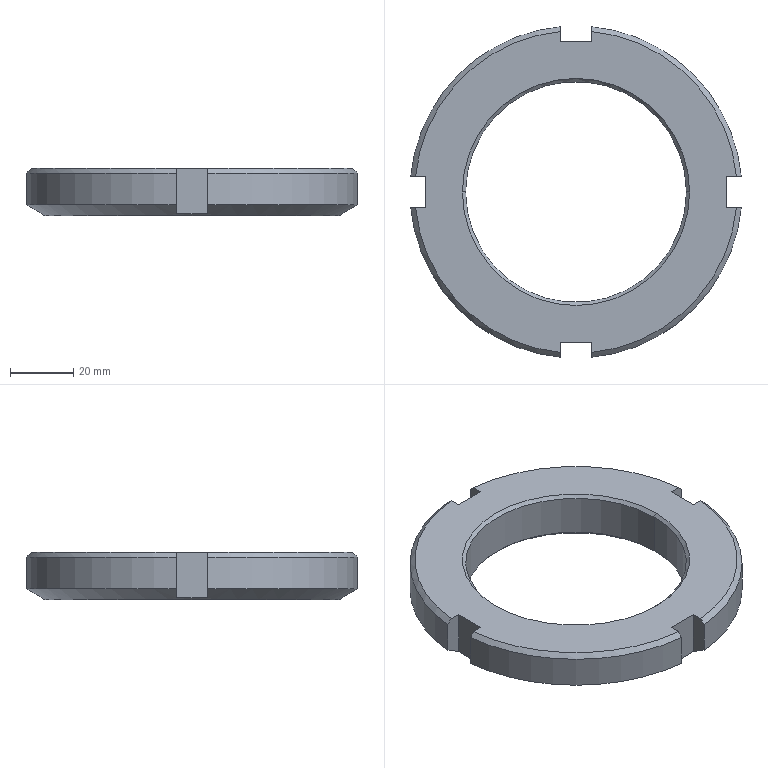Part | SolidWorks | features Chamfer 3, CirPattern 1, Cut 1, Extrusion 1 | 1 solid | 30 faces | box 104.523 x 104.523 x 15 mm | volume 66046 mm3 | plane 14 | cone 10 | cylinder 6 | commonest cylinder face diameters 105 x4 69.835 x2
STEP:
#1=CARTESIAN_POINT('',(-34.917,0.,14.));
#2=VERTEX_POINT('',#1);
#3=CARTESIAN_POINT('',(34.917,0.,14.));
#4=VERTEX_POINT('',#3);
#5=CARTESIAN_POINT('',(0.,0.,14.));
#6=DIRECTION('',(0.,0.,1.));
#7=DIRECTION('',(1.,0.,0.));
#8=AXIS2_PLACEMENT_3D('',#5,#6,#7);
#9=CIRCLE('',#8,34.917);
#10=EDGE_CURVE('',#2,#4,#9,.T.);
#11=ORIENTED_EDGE('',*,*,#10,.F.);
#12=CARTESIAN_POINT('',(-35.918,0.,15.));
#13=VERTEX_POINT('',#12);
#14=CARTESIAN_POINT('',(-34.917,0.,14.));
#15=DIRECTION('',(-0.7071,0.,0.7071));
#16=VECTOR('',#15,1000.);
#17=LINE('',#14,#16);
#18=EDGE_CURVE('',#2,#13,#17,.T.);
#19=ORIENTED_EDGE('',*,*,#18,.T.);
#20=CARTESIAN_POINT('',(35.918,0.,15.));
#21=VERTEX_POINT('',#20);
#22=CARTESIAN_POINT('',(0.,0.,15.));
#23=DIRECTION('',(0.,0.,-1.));
#24=DIRECTION('',(1.,0.,0.));
#25=AXIS2_PLACEMENT_3D('',#22,#23,#24);
#26=CIRCLE('',#25,35.918);
#27=EDGE_CURVE('',#21,#13,#26,.T.);
#28=ORIENTED_EDGE('',*,*,#27,.F.);
#29=CARTESIAN_POINT('',(34.917,0.,14.));
#30=DIRECTION('',(0.7071,0.,0.7071));
#31=VECTOR('',#30,1000.);
#32=LINE('',#29,#31);
#33=EDGE_CURVE('',#4,#21,#32,.T.);
#34=ORIENTED_EDGE('',*,*,#33,.F.);
#35=EDGE_LOOP('',(#11,#19,#28,#34));
#36=FACE_OUTER_BOUND('',#35,.T.);
#37=CARTESIAN_POINT('',(0.,0.,14.));
#38=DIRECTION('',(0.,0.,1.));
#39=DIRECTION('',(1.,0.,0.));
#40=AXIS2_PLACEMENT_3D('',#37,#38,#39);
#41=CONICAL_SURFACE('',#40,34.917,0.7854);
#42=ADVANCED_FACE('',(#36),#41,.F.);
#43=CARTESIAN_POINT('',(34.917,0.,1.));
#44=VERTEX_POINT('',#43);
#45=CARTESIAN_POINT('',(-34.917,0.,1.));
#46=VERTEX_POINT('',#45);
#47=CARTESIAN_POINT('',(0.,0.,1.));
#48=DIRECTION('',(0.,0.,-1.));
#49=DIRECTION('',(1.,0.,0.));
#50=AXIS2_PLACEMENT_3D('',#47,#48,#49);
#51=CIRCLE('',#50,34.917);
#52=EDGE_CURVE('',#44,#46,#51,.T.);
#53=ORIENTED_EDGE('',*,*,#52,.F.);
#54=CARTESIAN_POINT('',(35.918,0.,0.));
#55=VERTEX_POINT('',#54);
#56=CARTESIAN_POINT('',(35.918,0.,0.));
#57=DIRECTION('',(0.7071,0.,-0.7071));
#58=VECTOR('',#57,1000.);
#59=LINE('',#56,#58);
#60=EDGE_CURVE('',#44,#55,#59,.T.);
#61=ORIENTED_EDGE('',*,*,#60,.T.);
#62=CARTESIAN_POINT('',(-35.918,0.,0.));
#63=VERTEX_POINT('',#62);
#64=CARTESIAN_POINT('',(0.,0.,0.));
#65=DIRECTION('',(0.,0.,1.));
#66=DIRECTION('',(1.,0.,0.));
#67=AXIS2_PLACEMENT_3D('',#64,#65,#66);
#68=CIRCLE('',#67,35.918);
#69=EDGE_CURVE('',#63,#55,#68,.T.);
#70=ORIENTED_EDGE('',*,*,#69,.F.);
#71=CARTESIAN_POINT('',(-35.918,0.,0.));
#72=DIRECTION('',(-0.7071,0.,-0.7071));
#73=VECTOR('',#72,1000.);
#74=LINE('',#71,#73);
#75=EDGE_CURVE('',#46,#63,#74,.T.);
#76=ORIENTED_EDGE('',*,*,#75,.F.);
#77=EDGE_LOOP('',(#53,#61,#70,#76));
#78=FACE_OUTER_BOUND('',#77,.T.);
#79=CARTESIAN_POINT('',(0.,0.,0.));
#80=DIRECTION('',(0.,0.,-1.));
#81=DIRECTION('',(-1.,0.,0.));
#82=AXIS2_PLACEMENT_3D('',#79,#80,#81);
#83=CONICAL_SURFACE('',#82,35.918,0.7854);
#84=ADVANCED_FACE('',(#78),#83,.F.);
#85=CARTESIAN_POINT('',(-46.5,0.,0.));
#86=VERTEX_POINT('',#85);
#87=CARTESIAN_POINT('',(46.5,0.,0.));
#88=VERTEX_POINT('',#87);
#89=CARTESIAN_POINT('',(0.,0.,0.));
#90=DIRECTION('',(0.,0.,-1.));
#91=DIRECTION('',(1.,0.,0.));
#92=AXIS2_PLACEMENT_3D('',#89,#90,#91);
#93=CIRCLE('',#92,46.5);
#94=EDGE_CURVE('',#86,#88,#93,.T.);
#95=ORIENTED_EDGE('',*,*,#94,.F.);
#96=CARTESIAN_POINT('',(-47.511,0.,0.5839));
#97=VERTEX_POINT('',#96);
#98=CARTESIAN_POINT('',(-52.5,0.,3.464));
#99=DIRECTION('',(-0.866,0.,0.5));
#100=VECTOR('',#99,1000.);
#101=LINE('',#98,#100);
#102=EDGE_CURVE('',#86,#97,#101,.T.);
#103=ORIENTED_EDGE('',*,*,#102,.T.);
#104=CARTESIAN_POINT('',(-47.511,5.,0.7354));
#105=VERTEX_POINT('',#104);
#106=CARTESIAN_POINT('',(-47.511,5.,0.7354));
#107=CARTESIAN_POINT('',(-47.511,3.337,0.6349));
#108=CARTESIAN_POINT('',(-47.511,1.671,0.5839));
#109=CARTESIAN_POINT('',(-47.511,0.,0.5839));
#110=B_SPLINE_CURVE_WITH_KNOTS('',3,(#106,#107,#108,#109),.UNSPECIFIED.,.F.,.F.,(4,4),(0.01217,0.01717),.UNSPECIFIED.);
#111=EDGE_CURVE('',#105,#97,#110,.T.);
#112=ORIENTED_EDGE('',*,*,#111,.F.);
#113=CARTESIAN_POINT('',(-52.261,5.,3.464));
#114=VERTEX_POINT('',#113);
#115=CARTESIAN_POINT('',(-52.261,5.,3.464));
#116=CARTESIAN_POINT('',(-51.988,5.,3.307));
#117=CARTESIAN_POINT('',(-51.714,5.,3.15));
#118=CARTESIAN_POINT('',(-51.441,5.,2.993));
#119=CARTESIAN_POINT('',(-50.131,5.,2.24));
#120=CARTESIAN_POINT('',(-48.821,5.,1.488));
#121=CARTESIAN_POINT('',(-47.511,5.,0.7354));
#122=B_SPLINE_CURVE_WITH_KNOTS('',3,(#115,#116,#117,#118,#119,#120,#121),.UNSPECIFIED.,.F.,.F.,(4,3,4),(0.01027,0.01122,0.01575),.UNSPECIFIED.);
#123=EDGE_CURVE('',#114,#105,#122,.T.);
#124=ORIENTED_EDGE('',*,*,#123,.F.);
#125=CARTESIAN_POINT('',(-5.,52.261,3.464));
#126=VERTEX_POINT('',#125);
#127=CARTESIAN_POINT('',(0.,0.,3.464));
#128=DIRECTION('',(0.,0.,1.));
#129=DIRECTION('',(1.,0.,0.));
#130=AXIS2_PLACEMENT_3D('',#127,#128,#129);
#131=CIRCLE('',#130,52.5);
#132=EDGE_CURVE('',#126,#114,#131,.T.);
#133=ORIENTED_EDGE('',*,*,#132,.F.);
#134=CARTESIAN_POINT('',(-5.,47.511,0.7354));
#135=VERTEX_POINT('',#134);
#136=CARTESIAN_POINT('',(-5.,47.511,0.7354));
#137=CARTESIAN_POINT('',(-5.,47.679,0.8316));
#138=CARTESIAN_POINT('',(-5.,47.847,0.9279));
#139=CARTESIAN_POINT('',(-5.,48.014,1.024));
#140=CARTESIAN_POINT('',(-5.,49.43,1.837));
#141=CARTESIAN_POINT('',(-5.,50.846,2.651));
#142=CARTESIAN_POINT('',(-5.,52.261,3.464));
#143=B_SPLINE_CURVE_WITH_KNOTS('',3,(#136,#137,#138,#139,#140,#141,#142),.UNSPECIFIED.,.F.,.F.,(4,3,4),(0.01064,0.01122,0.01612),.UNSPECIFIED.);
#144=EDGE_CURVE('',#135,#126,#143,.T.);
#145=ORIENTED_EDGE('',*,*,#144,.F.);
#146=CARTESIAN_POINT('',(5.,47.511,0.7354));
#147=VERTEX_POINT('',#146);
#148=CARTESIAN_POINT('',(5.,47.511,0.7354));
#149=CARTESIAN_POINT('',(3.341,47.511,0.6351));
#150=CARTESIAN_POINT('',(1.678,47.511,0.5841));
#151=CARTESIAN_POINT('',(-0.8227,47.511,0.5838));
#152=CARTESIAN_POINT('',(-1.657,47.511,0.5964));
#153=CARTESIAN_POINT('',(-3.328,47.511,0.6469));
#154=CARTESIAN_POINT('',(-4.165,47.511,0.685));
#155=CARTESIAN_POINT('',(-5.,47.511,0.7354));
#156=B_SPLINE_CURVE_WITH_KNOTS('',3,(#148,#149,#150,#151,#152,#153,#154,#155),.UNSPECIFIED.,.F.,.F.,(4,2,2,4),(0.01217,0.01715,0.01965,0.02214),.UNSPECIFIED.);
#157=EDGE_CURVE('',#147,#135,#156,.T.);
#158=ORIENTED_EDGE('',*,*,#157,.F.);
#159=CARTESIAN_POINT('',(5.,52.261,3.464));
#160=VERTEX_POINT('',#159);
#161=CARTESIAN_POINT('',(5.,52.261,3.464));
#162=CARTESIAN_POINT('',(5.,50.846,2.651));
#163=CARTESIAN_POINT('',(5.,49.43,1.837));
#164=CARTESIAN_POINT('',(5.,48.014,1.024));
#165=CARTESIAN_POINT('',(5.,47.847,0.9279));
#166=CARTESIAN_POINT('',(5.,47.679,0.8316));
#167=CARTESIAN_POINT('',(5.,47.511,0.7354));
#168=B_SPLINE_CURVE_WITH_KNOTS('',3,(#161,#162,#163,#164,#165,#166,#167),.UNSPECIFIED.,.F.,.F.,(4,3,4),(0.006321,0.01122,0.0118),.UNSPECIFIED.);
#169=EDGE_CURVE('',#160,#147,#168,.T.);
#170=ORIENTED_EDGE('',*,*,#169,.F.);
#171=CARTESIAN_POINT('',(52.261,5.,3.464));
#172=VERTEX_POINT('',#171);
#173=CARTESIAN_POINT('',(0.,0.,3.464));
#174=DIRECTION('',(0.,0.,1.));
#175=DIRECTION('',(1.,0.,0.));
#176=AXIS2_PLACEMENT_3D('',#173,#174,#175);
#177=CIRCLE('',#176,52.5);
#178=EDGE_CURVE('',#172,#160,#177,.T.);
#179=ORIENTED_EDGE('',*,*,#178,.F.);
#180=CARTESIAN_POINT('',(47.511,5.,0.7354));
#181=VERTEX_POINT('',#180);
#182=CARTESIAN_POINT('',(47.511,5.,0.7354));
#183=CARTESIAN_POINT('',(47.679,5.,0.8316));
#184=CARTESIAN_POINT('',(47.847,5.,0.9279));
#185=CARTESIAN_POINT('',(48.014,5.,1.024));
#186=CARTESIAN_POINT('',(49.43,5.,1.837));
#187=CARTESIAN_POINT('',(50.846,5.,2.651));
#188=CARTESIAN_POINT('',(52.261,5.,3.464));
#189=B_SPLINE_CURVE_WITH_KNOTS('',3,(#182,#183,#184,#185,#186,#187,#188),.UNSPECIFIED.,.F.,.F.,(4,3,4),(0.01064,0.01122,0.01612),.UNSPECIFIED.);
#190=EDGE_CURVE('',#181,#172,#189,.T.);
#191=ORIENTED_EDGE('',*,*,#190,.F.);
#192=CARTESIAN_POINT('',(47.511,0.,0.5839));
#193=VERTEX_POINT('',#192);
#194=CARTESIAN_POINT('',(47.511,0.,0.5839));
#195=CARTESIAN_POINT('',(47.511,1.671,0.5839));
#196=CARTESIAN_POINT('',(47.511,3.337,0.6349));
#197=CARTESIAN_POINT('',(47.511,5.,0.7354));
#198=B_SPLINE_CURVE_WITH_KNOTS('',3,(#194,#195,#196,#197),.UNSPECIFIED.,.F.,.F.,(4,4),(0.0247,0.02971),.UNSPECIFIED.);
#199=EDGE_CURVE('',#193,#181,#198,.T.);
#200=ORIENTED_EDGE('',*,*,#199,.F.);
#201=CARTESIAN_POINT('',(52.5,0.,3.464));
#202=DIRECTION('',(0.866,0.,0.5));
#203=VECTOR('',#202,1000.);
#204=LINE('',#201,#203);
#205=EDGE_CURVE('',#88,#193,#204,.T.);
#206=ORIENTED_EDGE('',*,*,#205,.F.);
#207=EDGE_LOOP('',(#95,#103,#112,#124,#133,#145,#158,#170,#179,#191,#200,#206));
#208=FACE_OUTER_BOUND('',#207,.T.);
#209=CARTESIAN_POINT('',(0.,0.,3.464));
#210=DIRECTION('',(0.,0.,1.));
#211=DIRECTION('',(1.,0.,0.));
#212=AXIS2_PLACEMENT_3D('',#209,#210,#211);
#213=CONICAL_SURFACE('',#212,52.5,1.047);
#214=ADVANCED_FACE('',(#208),#213,.T.);
#215=ORIENTED_EDGE('',*,*,#10,.T.);
#216=CARTESIAN_POINT('',(34.917,0.,15.));
#217=DIRECTION('',(0.,0.,-1.));
#218=VECTOR('',#217,1000.);
#219=LINE('',#216,#218);
#220=EDGE_CURVE('',#4,#44,#219,.T.);
#221=ORIENTED_EDGE('',*,*,#220,.T.);
#222=ORIENTED_EDGE('',*,*,#52,.T.);
#223=CARTESIAN_POINT('',(-34.917,0.,15.));
#224=DIRECTION('',(0.,0.,-1.));
#225=VECTOR('',#224,1000.);
#226=LINE('',#223,#225);
#227=EDGE_CURVE('',#2,#46,#226,.T.);
#228=ORIENTED_EDGE('',*,*,#227,.F.);
#229=EDGE_LOOP('',(#215,#221,#222,#228));
#230=FACE_OUTER_BOUND('',#229,.T.);
#231=CARTESIAN_POINT('',(0.,0.,15.));
#232=DIRECTION('',(0.,0.,-1.));
#233=DIRECTION('',(-1.,0.,0.));
#234=AXIS2_PLACEMENT_3D('',#231,#232,#233);
#235=CYLINDRICAL_SURFACE('',#234,34.917);
#236=ADVANCED_FACE('',(#230),#235,.F.);
#237=CARTESIAN_POINT('',(5.,52.261,13.5));
#238=VERTEX_POINT('',#237);
#239=CARTESIAN_POINT('',(52.261,5.,13.5));
#240=VERTEX_POINT('',#239);
#241=CARTESIAN_POINT('',(0.,0.,13.5));
#242=DIRECTION('',(0.,0.,-1.));
#243=DIRECTION('',(1.,0.,0.));
#244=AXIS2_PLACEMENT_3D('',#241,#242,#243);
#245=CIRCLE('',#244,52.5);
#246=EDGE_CURVE('',#238,#240,#245,.T.);
#247=ORIENTED_EDGE('',*,*,#246,.T.);
#248=CARTESIAN_POINT('',(52.261,5.,0.));
#249=DIRECTION('',(0.,0.,1.));
#250=VECTOR('',#249,1000.);
#251=LINE('',#248,#250);
#252=EDGE_CURVE('',#172,#240,#251,.T.);
#253=ORIENTED_EDGE('',*,*,#252,.F.);
#254=ORIENTED_EDGE('',*,*,#178,.T.);
#255=CARTESIAN_POINT('',(5.,52.261,0.));
#256=DIRECTION('',(0.,0.,1.));
#257=VECTOR('',#256,1000.);
#258=LINE('',#255,#257);
#259=EDGE_CURVE('',#160,#238,#258,.T.);
#260=ORIENTED_EDGE('',*,*,#259,.T.);
#261=EDGE_LOOP('',(#247,#253,#254,#260));
#262=FACE_OUTER_BOUND('',#261,.T.);
#263=CARTESIAN_POINT('',(0.,0.,15.));
#264=DIRECTION('',(0.,0.,-1.));
#265=DIRECTION('',(-1.,0.,0.));
#266=AXIS2_PLACEMENT_3D('',#263,#264,#265);
#267=CYLINDRICAL_SURFACE('',#266,52.5);
#268=ADVANCED_FACE('',(#262),#267,.T.);
#269=CARTESIAN_POINT('',(50.754,5.,15.));
#270=VERTEX_POINT('',#269);
#271=CARTESIAN_POINT('',(52.261,5.,13.5));
#272=CARTESIAN_POINT('',(51.838,5.,13.921));
#273=CARTESIAN_POINT('',(51.415,5.,14.343));
#274=CARTESIAN_POINT('',(50.992,5.,14.764));
#275=CARTESIAN_POINT('',(50.912,5.,14.843));
#276=CARTESIAN_POINT('',(50.833,5.,14.921));
#277=CARTESIAN_POINT('',(50.754,5.,15.));
#278=B_SPLINE_CURVE_WITH_KNOTS('',3,(#271,#272,#273,#274,#275,#276,#277),.UNSPECIFIED.,.F.,.F.,(4,3,4),(0.00787,0.009662,0.009997),.UNSPECIFIED.);
#279=EDGE_CURVE('',#240,#270,#278,.T.);
#280=ORIENTED_EDGE('',*,*,#279,.F.);
#281=ORIENTED_EDGE('',*,*,#246,.F.);
#282=CARTESIAN_POINT('',(5.,50.754,15.));
#283=VERTEX_POINT('',#282);
#284=CARTESIAN_POINT('',(5.,50.754,15.));
#285=CARTESIAN_POINT('',(5.,50.833,14.921));
#286=CARTESIAN_POINT('',(5.,50.912,14.843));
#287=CARTESIAN_POINT('',(5.,50.992,14.764));
#288=CARTESIAN_POINT('',(5.,51.415,14.343));
#289=CARTESIAN_POINT('',(5.,51.838,13.921));
#290=CARTESIAN_POINT('',(5.,52.261,13.5));
#291=B_SPLINE_CURVE_WITH_KNOTS('',3,(#284,#285,#286,#287,#288,#289,#290),.UNSPECIFIED.,.F.,.F.,(4,3,4),(0.009327,0.009662,0.01145),.UNSPECIFIED.);
#292=EDGE_CURVE('',#283,#238,#291,.T.);
#293=ORIENTED_EDGE('',*,*,#292,.F.);
#294=CARTESIAN_POINT('',(0.,0.,15.));
#295=DIRECTION('',(0.,0.,1.));
#296=DIRECTION('',(1.,0.,0.));
#297=AXIS2_PLACEMENT_3D('',#294,#295,#296);
#298=CIRCLE('',#297,51.);
#299=EDGE_CURVE('',#270,#283,#298,.T.);
#300=ORIENTED_EDGE('',*,*,#299,.F.);
#301=EDGE_LOOP('',(#280,#281,#293,#300));
#302=FACE_OUTER_BOUND('',#301,.T.);
#303=CARTESIAN_POINT('',(0.,0.,15.));
#304=DIRECTION('',(0.,0.,-1.));
#305=DIRECTION('',(-1.,0.,0.));
#306=AXIS2_PLACEMENT_3D('',#303,#304,#305);
#307=CONICAL_SURFACE('',#306,51.,0.7854);
#308=ADVANCED_FACE('',(#302),#307,.T.);
#309=CARTESIAN_POINT('',(-52.261,5.,13.5));
#310=VERTEX_POINT('',#309);
#311=CARTESIAN_POINT('',(-5.,52.261,13.5));
#312=VERTEX_POINT('',#311);
#313=CARTESIAN_POINT('',(0.,0.,13.5));
#314=DIRECTION('',(0.,0.,-1.));
#315=DIRECTION('',(1.,0.,0.));
#316=AXIS2_PLACEMENT_3D('',#313,#314,#315);
#317=CIRCLE('',#316,52.5);
#318=EDGE_CURVE('',#310,#312,#317,.T.);
#319=ORIENTED_EDGE('',*,*,#318,.T.);
#320=CARTESIAN_POINT('',(-5.,52.261,0.));
#321=DIRECTION('',(0.,0.,1.));
#322=VECTOR('',#321,1000.);
#323=LINE('',#320,#322);
#324=EDGE_CURVE('',#126,#312,#323,.T.);
#325=ORIENTED_EDGE('',*,*,#324,.F.);
#326=ORIENTED_EDGE('',*,*,#132,.T.);
#327=CARTESIAN_POINT('',(-52.261,5.,0.));
#328=DIRECTION('',(0.,0.,1.));
#329=VECTOR('',#328,1000.);
#330=LINE('',#327,#329);
#331=EDGE_CURVE('',#114,#310,#330,.T.);
#332=ORIENTED_EDGE('',*,*,#331,.T.);
#333=EDGE_LOOP('',(#319,#325,#326,#332));
#334=FACE_OUTER_BOUND('',#333,.T.);
#335=CARTESIAN_POINT('',(0.,0.,15.));
#336=DIRECTION('',(0.,0.,-1.));
#337=DIRECTION('',(-1.,0.,0.));
#338=AXIS2_PLACEMENT_3D('',#335,#336,#337);
#339=CYLINDRICAL_SURFACE('',#338,52.5);
#340=ADVANCED_FACE('',(#334),#339,.T.);
#341=CARTESIAN_POINT('',(-5.,50.754,15.));
#342=VERTEX_POINT('',#341);
#343=CARTESIAN_POINT('',(-5.,52.261,13.5));
#344=CARTESIAN_POINT('',(-5.,51.838,13.921));
#345=CARTESIAN_POINT('',(-5.,51.415,14.343));
#346=CARTESIAN_POINT('',(-5.,50.992,14.764));
#347=CARTESIAN_POINT('',(-5.,50.912,14.843));
#348=CARTESIAN_POINT('',(-5.,50.833,14.921));
#349=CARTESIAN_POINT('',(-5.,50.754,15.));
#350=B_SPLINE_CURVE_WITH_KNOTS('',3,(#343,#344,#345,#346,#347,#348,#349),.UNSPECIFIED.,.F.,.F.,(4,3,4),(0.00787,0.009662,0.009997),.UNSPECIFIED.);
#351=EDGE_CURVE('',#312,#342,#350,.T.);
#352=ORIENTED_EDGE('',*,*,#351,.F.);
#353=ORIENTED_EDGE('',*,*,#318,.F.);
#354=CARTESIAN_POINT('',(-50.754,5.,15.));
#355=VERTEX_POINT('',#354);
#356=CARTESIAN_POINT('',(-50.754,5.,15.));
#357=CARTESIAN_POINT('',(-51.032,5.,14.723));
#358=CARTESIAN_POINT('',(-51.31,5.,14.447));
#359=CARTESIAN_POINT('',(-51.588,5.,14.17));
#360=CARTESIAN_POINT('',(-51.813,5.,13.947));
#361=CARTESIAN_POINT('',(-52.037,5.,13.723));
#362=CARTESIAN_POINT('',(-52.261,5.,13.5));
#363=B_SPLINE_CURVE_WITH_KNOTS('',3,(#356,#357,#358,#359,#360,#361,#362),.UNSPECIFIED.,.F.,.F.,(4,3,4),(0.008486,0.009662,0.01061),.UNSPECIFIED.);
#364=EDGE_CURVE('',#355,#310,#363,.T.);
#365=ORIENTED_EDGE('',*,*,#364,.F.);
#366=CARTESIAN_POINT('',(0.,0.,15.));
#367=DIRECTION('',(0.,0.,1.));
#368=DIRECTION('',(1.,0.,0.));
#369=AXIS2_PLACEMENT_3D('',#366,#367,#368);
#370=CIRCLE('',#369,51.);
#371=EDGE_CURVE('',#342,#355,#370,.T.);
#372=ORIENTED_EDGE('',*,*,#371,.F.);
#373=EDGE_LOOP('',(#352,#353,#365,#372));
#374=FACE_OUTER_BOUND('',#373,.T.);
#375=CARTESIAN_POINT('',(0.,0.,15.));
#376=DIRECTION('',(0.,0.,-1.));
#377=DIRECTION('',(-1.,0.,0.));
#378=AXIS2_PLACEMENT_3D('',#375,#376,#377);
#379=CONICAL_SURFACE('',#378,51.,0.7854);
#380=ADVANCED_FACE('',(#374),#379,.T.);
#381=CARTESIAN_POINT('',(-5.,-52.261,13.5));
#382=VERTEX_POINT('',#381);
#383=CARTESIAN_POINT('',(-52.261,-5.,13.5));
#384=VERTEX_POINT('',#383);
#385=CARTESIAN_POINT('',(0.,0.,13.5));
#386=DIRECTION('',(0.,0.,-1.));
#387=DIRECTION('',(1.,0.,0.));
#388=AXIS2_PLACEMENT_3D('',#385,#386,#387);
#389=CIRCLE('',#388,52.5);
#390=EDGE_CURVE('',#382,#384,#389,.T.);
#391=ORIENTED_EDGE('',*,*,#390,.T.);
#392=CARTESIAN_POINT('',(-52.261,-5.,3.464));
#393=VERTEX_POINT('',#392);
#394=CARTESIAN_POINT('',(-52.261,-5.,0.));
#395=DIRECTION('',(0.,0.,1.));
#396=VECTOR('',#395,1000.);
#397=LINE('',#394,#396);
#398=EDGE_CURVE('',#393,#384,#397,.T.);
#399=ORIENTED_EDGE('',*,*,#398,.F.);
#400=CARTESIAN_POINT('',(-5.,-52.261,3.464));
#401=VERTEX_POINT('',#400);
#402=CARTESIAN_POINT('',(0.,0.,3.464));
#403=DIRECTION('',(0.,0.,1.));
#404=DIRECTION('',(1.,0.,0.));
#405=AXIS2_PLACEMENT_3D('',#402,#403,#404);
#406=CIRCLE('',#405,52.5);
#407=EDGE_CURVE('',#393,#401,#406,.T.);
#408=ORIENTED_EDGE('',*,*,#407,.T.);
#409=CARTESIAN_POINT('',(-5.,-52.261,0.));
#410=DIRECTION('',(0.,0.,1.));
#411=VECTOR('',#410,1000.);
#412=LINE('',#409,#411);
#413=EDGE_CURVE('',#401,#382,#412,.T.);
#414=ORIENTED_EDGE('',*,*,#413,.T.);
#415=EDGE_LOOP('',(#391,#399,#408,#414));
#416=FACE_OUTER_BOUND('',#415,.T.);
#417=CARTESIAN_POINT('',(0.,0.,15.));
#418=DIRECTION('',(0.,0.,-1.));
#419=DIRECTION('',(-1.,0.,0.));
#420=AXIS2_PLACEMENT_3D('',#417,#418,#419);
#421=CYLINDRICAL_SURFACE('',#420,52.5);
#422=ADVANCED_FACE('',(#416),#421,.T.);
#423=CARTESIAN_POINT('',(-50.754,-5.,15.));
#424=VERTEX_POINT('',#423);
#425=CARTESIAN_POINT('',(-52.261,-5.,13.5));
#426=CARTESIAN_POINT('',(-52.037,-5.,13.723));
#427=CARTESIAN_POINT('',(-51.813,-5.,13.947));
#428=CARTESIAN_POINT('',(-51.588,-5.,14.17));
#429=CARTESIAN_POINT('',(-51.31,-5.,14.447));
#430=CARTESIAN_POINT('',(-51.032,-5.,14.723));
#431=CARTESIAN_POINT('',(-50.754,-5.,15.));
#432=B_SPLINE_CURVE_WITH_KNOTS('',3,(#425,#426,#427,#428,#429,#430,#431),.UNSPECIFIED.,.F.,.F.,(4,3,4),(0.008712,0.009662,0.01084),.UNSPECIFIED.);
#433=EDGE_CURVE('',#384,#424,#432,.T.);
#434=ORIENTED_EDGE('',*,*,#433,.F.);
#435=ORIENTED_EDGE('',*,*,#390,.F.);
#436=CARTESIAN_POINT('',(-5.,-50.754,15.));
#437=VERTEX_POINT('',#436);
#438=CARTESIAN_POINT('',(-5.,-50.754,15.));
#439=CARTESIAN_POINT('',(-5.,-51.032,14.723));
#440=CARTESIAN_POINT('',(-5.,-51.31,14.447));
#441=CARTESIAN_POINT('',(-5.,-51.588,14.17));
#442=CARTESIAN_POINT('',(-5.,-51.813,13.947));
#443=CARTESIAN_POINT('',(-5.,-52.037,13.723));
#444=CARTESIAN_POINT('',(-5.,-52.261,13.5));
#445=B_SPLINE_CURVE_WITH_KNOTS('',3,(#438,#439,#440,#441,#442,#443,#444),.UNSPECIFIED.,.F.,.F.,(4,3,4),(0.008486,0.009662,0.01061),.UNSPECIFIED.);
#446=EDGE_CURVE('',#437,#382,#445,.T.);
#447=ORIENTED_EDGE('',*,*,#446,.F.);
#448=CARTESIAN_POINT('',(0.,0.,15.));
#449=DIRECTION('',(0.,0.,1.));
#450=DIRECTION('',(1.,0.,0.));
#451=AXIS2_PLACEMENT_3D('',#448,#449,#450);
#452=CIRCLE('',#451,51.);
#453=EDGE_CURVE('',#424,#437,#452,.T.);
#454=ORIENTED_EDGE('',*,*,#453,.F.);
#455=EDGE_LOOP('',(#434,#435,#447,#454));
#456=FACE_OUTER_BOUND('',#455,.T.);
#457=CARTESIAN_POINT('',(0.,0.,15.));
#458=DIRECTION('',(0.,0.,-1.));
#459=DIRECTION('',(-1.,0.,0.));
#460=AXIS2_PLACEMENT_3D('',#457,#458,#459);
#461=CONICAL_SURFACE('',#460,51.,0.7854);
#462=ADVANCED_FACE('',(#456),#461,.T.);
#463=ORIENTED_EDGE('',*,*,#27,.T.);
#464=CARTESIAN_POINT('',(0.,0.,15.));
#465=DIRECTION('',(0.,0.,-1.));
#466=DIRECTION('',(1.,0.,0.));
#467=AXIS2_PLACEMENT_3D('',#464,#465,#466);
#468=CIRCLE('',#467,35.918);
#469=EDGE_CURVE('',#13,#21,#468,.T.);
#470=ORIENTED_EDGE('',*,*,#469,.T.);
#471=EDGE_LOOP('',(#463,#470));
#472=FACE_BOUND('',#471,.T.);
#473=CARTESIAN_POINT('',(47.511,5.,15.));
#474=VERTEX_POINT('',#473);
#475=CARTESIAN_POINT('',(47.511,5.,15.));
#476=DIRECTION('',(-1.,0.,0.));
#477=VECTOR('',#476,1000.);
#478=LINE('',#475,#477);
#479=EDGE_CURVE('',#270,#474,#478,.T.);
#480=ORIENTED_EDGE('',*,*,#479,.F.);
#481=ORIENTED_EDGE('',*,*,#299,.T.);
#482=CARTESIAN_POINT('',(5.,47.511,15.));
#483=VERTEX_POINT('',#482);
#484=CARTESIAN_POINT('',(5.,47.511,15.));
#485=DIRECTION('',(0.,1.,0.));
#486=VECTOR('',#485,1000.);
#487=LINE('',#484,#486);
#488=EDGE_CURVE('',#483,#283,#487,.T.);
#489=ORIENTED_EDGE('',*,*,#488,.F.);
#490=CARTESIAN_POINT('',(-5.,47.511,15.));
#491=VERTEX_POINT('',#490);
#492=CARTESIAN_POINT('',(5.,47.511,15.));
#493=DIRECTION('',(1.,0.,0.));
#494=VECTOR('',#493,1000.);
#495=LINE('',#492,#494);
#496=EDGE_CURVE('',#491,#483,#495,.T.);
#497=ORIENTED_EDGE('',*,*,#496,.F.);
#498=CARTESIAN_POINT('',(-5.,47.511,15.));
#499=DIRECTION('',(0.,-1.,0.));
#500=VECTOR('',#499,1000.);
#501=LINE('',#498,#500);
#502=EDGE_CURVE('',#342,#491,#501,.T.);
#503=ORIENTED_EDGE('',*,*,#502,.F.);
#504=ORIENTED_EDGE('',*,*,#371,.T.);
#505=CARTESIAN_POINT('',(-47.511,5.,15.));
#506=VERTEX_POINT('',#505);
#507=CARTESIAN_POINT('',(-47.511,5.,15.));
#508=DIRECTION('',(-1.,0.,0.));
#509=VECTOR('',#508,1000.);
#510=LINE('',#507,#509);
#511=EDGE_CURVE('',#506,#355,#510,.T.);
#512=ORIENTED_EDGE('',*,*,#511,.F.);
#513=CARTESIAN_POINT('',(-47.511,-5.,15.));
#514=VERTEX_POINT('',#513);
#515=CARTESIAN_POINT('',(-47.511,5.,15.));
#516=DIRECTION('',(0.,1.,0.));
#517=VECTOR('',#516,1000.);
#518=LINE('',#515,#517);
#519=EDGE_CURVE('',#514,#506,#518,.T.);
#520=ORIENTED_EDGE('',*,*,#519,.F.);
#521=CARTESIAN_POINT('',(-47.511,-5.,15.));
#522=DIRECTION('',(1.,0.,0.));
#523=VECTOR('',#522,1000.);
#524=LINE('',#521,#523);
#525=EDGE_CURVE('',#424,#514,#524,.T.);
#526=ORIENTED_EDGE('',*,*,#525,.F.);
#527=ORIENTED_EDGE('',*,*,#453,.T.);
#528=CARTESIAN_POINT('',(-5.,-47.511,15.));
#529=VERTEX_POINT('',#528);
#530=CARTESIAN_POINT('',(-5.,-47.511,15.));
#531=DIRECTION('',(0.,-1.,0.));
#532=VECTOR('',#531,1000.);
#533=LINE('',#530,#532);
#534=EDGE_CURVE('',#529,#437,#533,.T.);
#535=ORIENTED_EDGE('',*,*,#534,.F.);
#536=CARTESIAN_POINT('',(5.,-47.511,15.));
#537=VERTEX_POINT('',#536);
#538=CARTESIAN_POINT('',(-5.,-47.511,15.));
#539=DIRECTION('',(-1.,0.,0.));
#540=VECTOR('',#539,1000.);
#541=LINE('',#538,#540);
#542=EDGE_CURVE('',#537,#529,#541,.T.);
#543=ORIENTED_EDGE('',*,*,#542,.F.);
#544=CARTESIAN_POINT('',(5.,-50.754,15.));
#545=VERTEX_POINT('',#544);
#546=CARTESIAN_POINT('',(5.,-47.511,15.));
#547=DIRECTION('',(0.,1.,0.));
#548=VECTOR('',#547,1000.);
#549=LINE('',#546,#548);
#550=EDGE_CURVE('',#545,#537,#549,.T.);
#551=ORIENTED_EDGE('',*,*,#550,.F.);
#552=CARTESIAN_POINT('',(50.754,-5.,15.));
#553=VERTEX_POINT('',#552);
#554=CARTESIAN_POINT('',(0.,0.,15.));
#555=DIRECTION('',(0.,0.,1.));
#556=DIRECTION('',(1.,0.,0.));
#557=AXIS2_PLACEMENT_3D('',#554,#555,#556);
#558=CIRCLE('',#557,51.);
#559=EDGE_CURVE('',#545,#553,#558,.T.);
#560=ORIENTED_EDGE('',*,*,#559,.T.);
#561=CARTESIAN_POINT('',(47.511,-5.,15.));
#562=VERTEX_POINT('',#561);
#563=CARTESIAN_POINT('',(47.511,-5.,15.));
#564=DIRECTION('',(1.,0.,0.));
#565=VECTOR('',#564,1000.);
#566=LINE('',#563,#565);
#567=EDGE_CURVE('',#562,#553,#566,.T.);
#568=ORIENTED_EDGE('',*,*,#567,.F.);
#569=CARTESIAN_POINT('',(47.511,-5.,15.));
#570=DIRECTION('',(0.,-1.,0.));
#571=VECTOR('',#570,1000.);
#572=LINE('',#569,#571);
#573=EDGE_CURVE('',#474,#562,#572,.T.);
#574=ORIENTED_EDGE('',*,*,#573,.F.);
#575=EDGE_LOOP('',(#480,#481,#489,#497,#503,#504,#512,#520,#526,#527,#535,#543,#551,#560,#568,#574));
#576=FACE_OUTER_BOUND('',#575,.T.);
#577=CARTESIAN_POINT('',(0.,0.,15.));
#578=DIRECTION('',(0.,0.,1.));
#579=DIRECTION('',(1.,0.,0.));
#580=AXIS2_PLACEMENT_3D('',#577,#578,#579);
#581=PLANE('',#580);
#582=ADVANCED_FACE('',(#472,#576),#581,.T.);
#583=ORIENTED_EDGE('',*,*,#69,.T.);
#584=CARTESIAN_POINT('',(0.,0.,0.));
#585=DIRECTION('',(0.,0.,1.));
#586=DIRECTION('',(1.,0.,0.));
#587=AXIS2_PLACEMENT_3D('',#584,#585,#586);
#588=CIRCLE('',#587,35.918);
#589=EDGE_CURVE('',#55,#63,#588,.T.);
#590=ORIENTED_EDGE('',*,*,#589,.T.);
#591=EDGE_LOOP('',(#583,#590));
#592=FACE_BOUND('',#591,.T.);
#593=CARTESIAN_POINT('',(0.,0.,0.));
#594=DIRECTION('',(0.,0.,-1.));
#595=DIRECTION('',(1.,0.,0.));
#596=AXIS2_PLACEMENT_3D('',#593,#594,#595);
#597=CIRCLE('',#596,46.5);
#598=EDGE_CURVE('',#88,#86,#597,.T.);
#599=ORIENTED_EDGE('',*,*,#598,.T.);
#600=ORIENTED_EDGE('',*,*,#94,.T.);
#601=EDGE_LOOP('',(#599,#600));
#602=FACE_OUTER_BOUND('',#601,.T.);
#603=CARTESIAN_POINT('',(0.,0.,0.));
#604=DIRECTION('',(0.,0.,1.));
#605=DIRECTION('',(1.,0.,0.));
#606=AXIS2_PLACEMENT_3D('',#603,#604,#605);
#607=PLANE('',#606);
#608=ADVANCED_FACE('',(#592,#602),#607,.F.);
#609=CARTESIAN_POINT('',(5.,-52.261,3.464));
#610=VERTEX_POINT('',#609);
#611=CARTESIAN_POINT('',(52.261,-5.,3.464));
#612=VERTEX_POINT('',#611);
#613=CARTESIAN_POINT('',(0.,0.,3.464));
#614=DIRECTION('',(0.,0.,1.));
#615=DIRECTION('',(1.,0.,0.));
#616=AXIS2_PLACEMENT_3D('',#613,#614,#615);
#617=CIRCLE('',#616,52.5);
#618=EDGE_CURVE('',#610,#612,#617,.T.);
#619=ORIENTED_EDGE('',*,*,#618,.T.);
#620=CARTESIAN_POINT('',(52.261,-5.,13.5));
#621=VERTEX_POINT('',#620);
#622=CARTESIAN_POINT('',(52.261,-5.,0.));
#623=DIRECTION('',(0.,0.,1.));
#624=VECTOR('',#623,1000.);
#625=LINE('',#622,#624);
#626=EDGE_CURVE('',#612,#621,#625,.T.);
#627=ORIENTED_EDGE('',*,*,#626,.T.);
#628=CARTESIAN_POINT('',(5.,-52.261,13.5));
#629=VERTEX_POINT('',#628);
#630=CARTESIAN_POINT('',(0.,0.,13.5));
#631=DIRECTION('',(0.,0.,-1.));
#632=DIRECTION('',(1.,0.,0.));
#633=AXIS2_PLACEMENT_3D('',#630,#631,#632);
#634=CIRCLE('',#633,52.5);
#635=EDGE_CURVE('',#621,#629,#634,.T.);
#636=ORIENTED_EDGE('',*,*,#635,.T.);
#637=CARTESIAN_POINT('',(5.,-52.261,0.));
#638=DIRECTION('',(0.,0.,1.));
#639=VECTOR('',#638,1000.);
#640=LINE('',#637,#639);
#641=EDGE_CURVE('',#610,#629,#640,.T.);
#642=ORIENTED_EDGE('',*,*,#641,.F.);
#643=EDGE_LOOP('',(#619,#627,#636,#642));
#644=FACE_OUTER_BOUND('',#643,.T.);
#645=CARTESIAN_POINT('',(0.,0.,15.));
#646=DIRECTION('',(0.,0.,-1.));
#647=DIRECTION('',(-1.,0.,0.));
#648=AXIS2_PLACEMENT_3D('',#645,#646,#647);
#649=CYLINDRICAL_SURFACE('',#648,52.5);
#650=ADVANCED_FACE('',(#644),#649,.T.);
#651=ORIENTED_EDGE('',*,*,#220,.F.);
#652=CARTESIAN_POINT('',(0.,0.,14.));
#653=DIRECTION('',(0.,0.,1.));
#654=DIRECTION('',(1.,0.,0.));
#655=AXIS2_PLACEMENT_3D('',#652,#653,#654);
#656=CIRCLE('',#655,34.917);
#657=EDGE_CURVE('',#4,#2,#656,.T.);
#658=ORIENTED_EDGE('',*,*,#657,.T.);
#659=ORIENTED_EDGE('',*,*,#227,.T.);
#660=CARTESIAN_POINT('',(0.,0.,1.));
#661=DIRECTION('',(0.,0.,-1.));
#662=DIRECTION('',(1.,0.,0.));
#663=AXIS2_PLACEMENT_3D('',#660,#661,#662);
#664=CIRCLE('',#663,34.917);
#665=EDGE_CURVE('',#46,#44,#664,.T.);
#666=ORIENTED_EDGE('',*,*,#665,.T.);
#667=EDGE_LOOP('',(#651,#658,#659,#666));
#668=FACE_OUTER_BOUND('',#667,.T.);
#669=CARTESIAN_POINT('',(0.,0.,15.));
#670=DIRECTION('',(0.,0.,-1.));
#671=DIRECTION('',(-1.,0.,0.));
#672=AXIS2_PLACEMENT_3D('',#669,#670,#671);
#673=CYLINDRICAL_SURFACE('',#672,34.917);
#674=ADVANCED_FACE('',(#668),#673,.F.);
#675=CARTESIAN_POINT('',(50.754,-5.,15.));
#676=CARTESIAN_POINT('',(50.833,-5.,14.921));
#677=CARTESIAN_POINT('',(50.912,-5.,14.843));
#678=CARTESIAN_POINT('',(50.992,-5.,14.764));
#679=CARTESIAN_POINT('',(51.415,-5.,14.343));
#680=CARTESIAN_POINT('',(51.838,-5.,13.921));
#681=CARTESIAN_POINT('',(52.261,-5.,13.5));
#682=B_SPLINE_CURVE_WITH_KNOTS('',3,(#675,#676,#677,#678,#679,#680,#681),.UNSPECIFIED.,.F.,.F.,(4,3,4),(0.009327,0.009662,0.01145),.UNSPECIFIED.);
#683=EDGE_CURVE('',#553,#621,#682,.T.);
#684=ORIENTED_EDGE('',*,*,#683,.F.);
#685=ORIENTED_EDGE('',*,*,#559,.F.);
#686=CARTESIAN_POINT('',(5.,-52.261,13.5));
#687=CARTESIAN_POINT('',(5.,-52.037,13.723));
#688=CARTESIAN_POINT('',(5.,-51.813,13.947));
#689=CARTESIAN_POINT('',(5.,-51.588,14.17));
#690=CARTESIAN_POINT('',(5.,-51.31,14.447));
#691=CARTESIAN_POINT('',(5.,-51.032,14.723));
#692=CARTESIAN_POINT('',(5.,-50.754,15.));
#693=B_SPLINE_CURVE_WITH_KNOTS('',3,(#686,#687,#688,#689,#690,#691,#692),.UNSPECIFIED.,.F.,.F.,(4,3,4),(0.008712,0.009662,0.01084),.UNSPECIFIED.);
#694=EDGE_CURVE('',#629,#545,#693,.T.);
#695=ORIENTED_EDGE('',*,*,#694,.F.);
#696=ORIENTED_EDGE('',*,*,#635,.F.);
#697=EDGE_LOOP('',(#684,#685,#695,#696));
#698=FACE_OUTER_BOUND('',#697,.T.);
#699=CARTESIAN_POINT('',(0.,0.,15.));
#700=DIRECTION('',(0.,0.,-1.));
#701=DIRECTION('',(-1.,0.,0.));
#702=AXIS2_PLACEMENT_3D('',#699,#700,#701);
#703=CONICAL_SURFACE('',#702,51.,0.7854);
#704=ADVANCED_FACE('',(#698),#703,.T.);
#705=ORIENTED_EDGE('',*,*,#102,.F.);
#706=ORIENTED_EDGE('',*,*,#598,.F.);
#707=ORIENTED_EDGE('',*,*,#205,.T.);
#708=CARTESIAN_POINT('',(47.511,-5.,0.7354));
#709=VERTEX_POINT('',#708);
#710=CARTESIAN_POINT('',(47.511,-5.,0.7354));
#711=CARTESIAN_POINT('',(47.511,-4.167,0.6851));
#712=CARTESIAN_POINT('',(47.511,-3.332,0.6471));
#713=CARTESIAN_POINT('',(47.511,-1.664,0.5965));
#714=CARTESIAN_POINT('',(47.511,-0.8317,0.5839));
#715=CARTESIAN_POINT('',(47.511,0.,0.5839));
#716=B_SPLINE_CURVE_WITH_KNOTS('',3,(#710,#711,#712,#713,#714,#715),.UNSPECIFIED.,.F.,.F.,(4,2,4),(0.01972,0.02221,0.0247),.UNSPECIFIED.);
#717=EDGE_CURVE('',#709,#193,#716,.T.);
#718=ORIENTED_EDGE('',*,*,#717,.F.);
#719=CARTESIAN_POINT('',(52.261,-5.,3.464));
#720=CARTESIAN_POINT('',(50.846,-5.,2.651));
#721=CARTESIAN_POINT('',(49.43,-5.,1.837));
#722=CARTESIAN_POINT('',(48.014,-5.,1.024));
#723=CARTESIAN_POINT('',(47.847,-5.,0.9279));
#724=CARTESIAN_POINT('',(47.679,-5.,0.8316));
#725=CARTESIAN_POINT('',(47.511,-5.,0.7354));
#726=B_SPLINE_CURVE_WITH_KNOTS('',3,(#719,#720,#721,#722,#723,#724,#725),.UNSPECIFIED.,.F.,.F.,(4,3,4),(0.006321,0.01122,0.0118),.UNSPECIFIED.);
#727=EDGE_CURVE('',#612,#709,#726,.T.);
#728=ORIENTED_EDGE('',*,*,#727,.F.);
#729=ORIENTED_EDGE('',*,*,#618,.F.);
#730=CARTESIAN_POINT('',(5.,-47.511,0.7354));
#731=VERTEX_POINT('',#730);
#732=CARTESIAN_POINT('',(5.,-47.511,0.7354));
#733=CARTESIAN_POINT('',(5.,-48.821,1.488));
#734=CARTESIAN_POINT('',(5.,-50.131,2.24));
#735=CARTESIAN_POINT('',(5.,-51.441,2.993));
#736=CARTESIAN_POINT('',(5.,-51.714,3.15));
#737=CARTESIAN_POINT('',(5.,-51.988,3.307));
#738=CARTESIAN_POINT('',(5.,-52.261,3.464));
#739=B_SPLINE_CURVE_WITH_KNOTS('',3,(#732,#733,#734,#735,#736,#737,#738),.UNSPECIFIED.,.F.,.F.,(4,3,4),(0.006688,0.01122,0.01217),.UNSPECIFIED.);
#740=EDGE_CURVE('',#731,#610,#739,.T.);
#741=ORIENTED_EDGE('',*,*,#740,.F.);
#742=CARTESIAN_POINT('',(-5.,-47.511,0.7354));
#743=VERTEX_POINT('',#742);
#744=CARTESIAN_POINT('',(-5.,-47.511,0.7354));
#745=CARTESIAN_POINT('',(-4.165,-47.511,0.685));
#746=CARTESIAN_POINT('',(-3.328,-47.511,0.6469));
#747=CARTESIAN_POINT('',(-1.657,-47.511,0.5964));
#748=CARTESIAN_POINT('',(-0.8227,-47.511,0.5838));
#749=CARTESIAN_POINT('',(1.678,-47.511,0.5841));
#750=CARTESIAN_POINT('',(3.341,-47.511,0.6351));
#751=CARTESIAN_POINT('',(5.,-47.511,0.7354));
#752=B_SPLINE_CURVE_WITH_KNOTS('',3,(#744,#745,#746,#747,#748,#749,#750,#751),.UNSPECIFIED.,.F.,.F.,(4,2,2,4),(0.01972,0.02222,0.02472,0.02971),.UNSPECIFIED.);
#753=EDGE_CURVE('',#743,#731,#752,.T.);
#754=ORIENTED_EDGE('',*,*,#753,.F.);
#755=CARTESIAN_POINT('',(-5.,-52.261,3.464));
#756=CARTESIAN_POINT('',(-5.,-51.988,3.307));
#757=CARTESIAN_POINT('',(-5.,-51.714,3.15));
#758=CARTESIAN_POINT('',(-5.,-51.441,2.993));
#759=CARTESIAN_POINT('',(-5.,-50.131,2.24));
#760=CARTESIAN_POINT('',(-5.,-48.821,1.488));
#761=CARTESIAN_POINT('',(-5.,-47.511,0.7354));
#762=B_SPLINE_CURVE_WITH_KNOTS('',3,(#755,#756,#757,#758,#759,#760,#761),.UNSPECIFIED.,.F.,.F.,(4,3,4),(0.01027,0.01122,0.01575),.UNSPECIFIED.);
#763=EDGE_CURVE('',#401,#743,#762,.T.);
#764=ORIENTED_EDGE('',*,*,#763,.F.);
#765=ORIENTED_EDGE('',*,*,#407,.F.);
#766=CARTESIAN_POINT('',(-47.511,-5.,0.7354));
#767=VERTEX_POINT('',#766);
#768=CARTESIAN_POINT('',(-47.511,-5.,0.7354));
#769=CARTESIAN_POINT('',(-48.821,-5.,1.488));
#770=CARTESIAN_POINT('',(-50.131,-5.,2.24));
#771=CARTESIAN_POINT('',(-51.441,-5.,2.993));
#772=CARTESIAN_POINT('',(-51.714,-5.,3.15));
#773=CARTESIAN_POINT('',(-51.988,-5.,3.307));
#774=CARTESIAN_POINT('',(-52.261,-5.,3.464));
#775=B_SPLINE_CURVE_WITH_KNOTS('',3,(#768,#769,#770,#771,#772,#773,#774),.UNSPECIFIED.,.F.,.F.,(4,3,4),(0.006688,0.01122,0.01217),.UNSPECIFIED.);
#776=EDGE_CURVE('',#767,#393,#775,.T.);
#777=ORIENTED_EDGE('',*,*,#776,.F.);
#778=CARTESIAN_POINT('',(-47.511,0.,0.5839));
#779=CARTESIAN_POINT('',(-47.511,-0.8317,0.5839));
#780=CARTESIAN_POINT('',(-47.511,-1.664,0.5965));
#781=CARTESIAN_POINT('',(-47.511,-3.332,0.6471));
#782=CARTESIAN_POINT('',(-47.511,-4.167,0.6851));
#783=CARTESIAN_POINT('',(-47.511,-5.,0.7354));
#784=B_SPLINE_CURVE_WITH_KNOTS('',3,(#778,#779,#780,#781,#782,#783),.UNSPECIFIED.,.F.,.F.,(4,2,4),(0.01717,0.01965,0.02214),.UNSPECIFIED.);
#785=EDGE_CURVE('',#97,#767,#784,.T.);
#786=ORIENTED_EDGE('',*,*,#785,.F.);
#787=EDGE_LOOP('',(#705,#706,#707,#718,#728,#729,#741,#754,#764,#765,#777,#786));
#788=FACE_OUTER_BOUND('',#787,.T.);
#789=CARTESIAN_POINT('',(0.,0.,3.464));
#790=DIRECTION('',(0.,0.,1.));
#791=DIRECTION('',(1.,0.,0.));
#792=AXIS2_PLACEMENT_3D('',#789,#790,#791);
#793=CONICAL_SURFACE('',#792,52.5,1.047);
#794=ADVANCED_FACE('',(#788),#793,.T.);
#795=ORIENTED_EDGE('',*,*,#753,.T.);
#796=CARTESIAN_POINT('',(5.,-47.511,0.));
#797=DIRECTION('',(0.,0.,1.));
#798=VECTOR('',#797,1000.);
#799=LINE('',#796,#798);
#800=EDGE_CURVE('',#731,#537,#799,.T.);
#801=ORIENTED_EDGE('',*,*,#800,.T.);
#802=ORIENTED_EDGE('',*,*,#542,.T.);
#803=CARTESIAN_POINT('',(-5.,-47.511,0.));
#804=DIRECTION('',(0.,0.,1.));
#805=VECTOR('',#804,1000.);
#806=LINE('',#803,#805);
#807=EDGE_CURVE('',#743,#529,#806,.T.);
#808=ORIENTED_EDGE('',*,*,#807,.F.);
#809=EDGE_LOOP('',(#795,#801,#802,#808));
#810=FACE_OUTER_BOUND('',#809,.T.);
#811=CARTESIAN_POINT('',(-5.,-47.511,0.));
#812=DIRECTION('',(0.,1.,0.));
#813=DIRECTION('',(0.,0.,1.));
#814=AXIS2_PLACEMENT_3D('',#811,#812,#813);
#815=PLANE('',#814);
#816=ADVANCED_FACE('',(#810),#815,.F.);
#817=ORIENTED_EDGE('',*,*,#694,.T.);
#818=ORIENTED_EDGE('',*,*,#550,.T.);
#819=ORIENTED_EDGE('',*,*,#800,.F.);
#820=ORIENTED_EDGE('',*,*,#740,.T.);
#821=ORIENTED_EDGE('',*,*,#641,.T.);
#822=EDGE_LOOP('',(#817,#818,#819,#820,#821));
#823=FACE_OUTER_BOUND('',#822,.T.);
#824=CARTESIAN_POINT('',(5.,-47.511,0.));
#825=DIRECTION('',(1.,0.,0.));
#826=DIRECTION('',(0.,1.,0.));
#827=AXIS2_PLACEMENT_3D('',#824,#825,#826);
#828=PLANE('',#827);
#829=ADVANCED_FACE('',(#823),#828,.F.);
#830=ORIENTED_EDGE('',*,*,#446,.T.);
#831=ORIENTED_EDGE('',*,*,#413,.F.);
#832=ORIENTED_EDGE('',*,*,#763,.T.);
#833=ORIENTED_EDGE('',*,*,#807,.T.);
#834=ORIENTED_EDGE('',*,*,#534,.T.);
#835=EDGE_LOOP('',(#830,#831,#832,#833,#834));
#836=FACE_OUTER_BOUND('',#835,.T.);
#837=CARTESIAN_POINT('',(-5.,-47.511,0.));
#838=DIRECTION('',(-1.,0.,0.));
#839=DIRECTION('',(0.,-1.,0.));
#840=AXIS2_PLACEMENT_3D('',#837,#838,#839);
#841=PLANE('',#840);
#842=ADVANCED_FACE('',(#836),#841,.F.);
#843=ORIENTED_EDGE('',*,*,#111,.T.);
#844=ORIENTED_EDGE('',*,*,#785,.T.);
#845=CARTESIAN_POINT('',(-47.511,-5.,0.));
#846=DIRECTION('',(0.,0.,1.));
#847=VECTOR('',#846,1000.);
#848=LINE('',#845,#847);
#849=EDGE_CURVE('',#767,#514,#848,.T.);
#850=ORIENTED_EDGE('',*,*,#849,.T.);
#851=ORIENTED_EDGE('',*,*,#519,.T.);
#852=CARTESIAN_POINT('',(-47.511,5.,0.));
#853=DIRECTION('',(0.,0.,1.));
#854=VECTOR('',#853,1000.);
#855=LINE('',#852,#854);
#856=EDGE_CURVE('',#105,#506,#855,.T.);
#857=ORIENTED_EDGE('',*,*,#856,.F.);
#858=EDGE_LOOP('',(#843,#844,#850,#851,#857));
#859=FACE_OUTER_BOUND('',#858,.T.);
#860=CARTESIAN_POINT('',(-47.511,5.,0.));
#861=DIRECTION('',(1.,0.,0.));
#862=DIRECTION('',(0.,1.,0.));
#863=AXIS2_PLACEMENT_3D('',#860,#861,#862);
#864=PLANE('',#863);
#865=ADVANCED_FACE('',(#859),#864,.F.);
#866=ORIENTED_EDGE('',*,*,#433,.T.);
#867=ORIENTED_EDGE('',*,*,#525,.T.);
#868=ORIENTED_EDGE('',*,*,#849,.F.);
#869=ORIENTED_EDGE('',*,*,#776,.T.);
#870=ORIENTED_EDGE('',*,*,#398,.T.);
#871=EDGE_LOOP('',(#866,#867,#868,#869,#870));
#872=FACE_OUTER_BOUND('',#871,.T.);
#873=CARTESIAN_POINT('',(-47.511,-5.,0.));
#874=DIRECTION('',(0.,-1.,0.));
#875=DIRECTION('',(1.,0.,0.));
#876=AXIS2_PLACEMENT_3D('',#873,#874,#875);
#877=PLANE('',#876);
#878=ADVANCED_FACE('',(#872),#877,.F.);
#879=ORIENTED_EDGE('',*,*,#364,.T.);
#880=ORIENTED_EDGE('',*,*,#331,.F.);
#881=ORIENTED_EDGE('',*,*,#123,.T.);
#882=ORIENTED_EDGE('',*,*,#856,.T.);
#883=ORIENTED_EDGE('',*,*,#511,.T.);
#884=EDGE_LOOP('',(#879,#880,#881,#882,#883));
#885=FACE_OUTER_BOUND('',#884,.T.);
#886=CARTESIAN_POINT('',(-47.511,5.,0.));
#887=DIRECTION('',(0.,1.,0.));
#888=DIRECTION('',(-1.,0.,0.));
#889=AXIS2_PLACEMENT_3D('',#886,#887,#888);
#890=PLANE('',#889);
#891=ADVANCED_FACE('',(#885),#890,.F.);
#892=ORIENTED_EDGE('',*,*,#157,.T.);
#893=CARTESIAN_POINT('',(-5.,47.511,0.));
#894=DIRECTION('',(0.,0.,1.));
#895=VECTOR('',#894,1000.);
#896=LINE('',#893,#895);
#897=EDGE_CURVE('',#135,#491,#896,.T.);
#898=ORIENTED_EDGE('',*,*,#897,.T.);
#899=ORIENTED_EDGE('',*,*,#496,.T.);
#900=CARTESIAN_POINT('',(5.,47.511,0.));
#901=DIRECTION('',(0.,0.,1.));
#902=VECTOR('',#901,1000.);
#903=LINE('',#900,#902);
#904=EDGE_CURVE('',#147,#483,#903,.T.);
#905=ORIENTED_EDGE('',*,*,#904,.F.);
#906=EDGE_LOOP('',(#892,#898,#899,#905));
#907=FACE_OUTER_BOUND('',#906,.T.);
#908=CARTESIAN_POINT('',(5.,47.511,0.));
#909=DIRECTION('',(0.,-1.,0.));
#910=DIRECTION('',(1.,0.,0.));
#911=AXIS2_PLACEMENT_3D('',#908,#909,#910);
#912=PLANE('',#911);
#913=ADVANCED_FACE('',(#907),#912,.F.);
#914=ORIENTED_EDGE('',*,*,#351,.T.);
#915=ORIENTED_EDGE('',*,*,#502,.T.);
#916=ORIENTED_EDGE('',*,*,#897,.F.);
#917=ORIENTED_EDGE('',*,*,#144,.T.);
#918=ORIENTED_EDGE('',*,*,#324,.T.);
#919=EDGE_LOOP('',(#914,#915,#916,#917,#918));
#920=FACE_OUTER_BOUND('',#919,.T.);
#921=CARTESIAN_POINT('',(-5.,47.511,0.));
#922=DIRECTION('',(-1.,0.,0.));
#923=DIRECTION('',(0.,-1.,0.));
#924=AXIS2_PLACEMENT_3D('',#921,#922,#923);
#925=PLANE('',#924);
#926=ADVANCED_FACE('',(#920),#925,.F.);
#927=ORIENTED_EDGE('',*,*,#292,.T.);
#928=ORIENTED_EDGE('',*,*,#259,.F.);
#929=ORIENTED_EDGE('',*,*,#169,.T.);
#930=ORIENTED_EDGE('',*,*,#904,.T.);
#931=ORIENTED_EDGE('',*,*,#488,.T.);
#932=EDGE_LOOP('',(#927,#928,#929,#930,#931));
#933=FACE_OUTER_BOUND('',#932,.T.);
#934=CARTESIAN_POINT('',(5.,47.511,0.));
#935=DIRECTION('',(1.,0.,0.));
#936=DIRECTION('',(0.,1.,0.));
#937=AXIS2_PLACEMENT_3D('',#934,#935,#936);
#938=PLANE('',#937);
#939=ADVANCED_FACE('',(#933),#938,.F.);
#940=ORIENTED_EDGE('',*,*,#717,.T.);
#941=ORIENTED_EDGE('',*,*,#199,.T.);
#942=CARTESIAN_POINT('',(47.511,5.,0.));
#943=DIRECTION('',(0.,0.,1.));
#944=VECTOR('',#943,1000.);
#945=LINE('',#942,#944);
#946=EDGE_CURVE('',#181,#474,#945,.T.);
#947=ORIENTED_EDGE('',*,*,#946,.T.);
#948=ORIENTED_EDGE('',*,*,#573,.T.);
#949=CARTESIAN_POINT('',(47.511,-5.,0.));
#950=DIRECTION('',(0.,0.,1.));
#951=VECTOR('',#950,1000.);
#952=LINE('',#949,#951);
#953=EDGE_CURVE('',#709,#562,#952,.T.);
#954=ORIENTED_EDGE('',*,*,#953,.F.);
#955=EDGE_LOOP('',(#940,#941,#947,#948,#954));
#956=FACE_OUTER_BOUND('',#955,.T.);
#957=CARTESIAN_POINT('',(47.511,-5.,0.));
#958=DIRECTION('',(-1.,0.,0.));
#959=DIRECTION('',(0.,-1.,0.));
#960=AXIS2_PLACEMENT_3D('',#957,#958,#959);
#961=PLANE('',#960);
#962=ADVANCED_FACE('',(#956),#961,.F.);
#963=ORIENTED_EDGE('',*,*,#279,.T.);
#964=ORIENTED_EDGE('',*,*,#479,.T.);
#965=ORIENTED_EDGE('',*,*,#946,.F.);
#966=ORIENTED_EDGE('',*,*,#190,.T.);
#967=ORIENTED_EDGE('',*,*,#252,.T.);
#968=EDGE_LOOP('',(#963,#964,#965,#966,#967));
#969=FACE_OUTER_BOUND('',#968,.T.);
#970=CARTESIAN_POINT('',(47.511,5.,0.));
#971=DIRECTION('',(0.,1.,0.));
#972=DIRECTION('',(-1.,0.,0.));
#973=AXIS2_PLACEMENT_3D('',#970,#971,#972);
#974=PLANE('',#973);
#975=ADVANCED_FACE('',(#969),#974,.F.);
#976=ORIENTED_EDGE('',*,*,#683,.T.);
#977=ORIENTED_EDGE('',*,*,#626,.F.);
#978=ORIENTED_EDGE('',*,*,#727,.T.);
#979=ORIENTED_EDGE('',*,*,#953,.T.);
#980=ORIENTED_EDGE('',*,*,#567,.T.);
#981=EDGE_LOOP('',(#976,#977,#978,#979,#980));
#982=FACE_OUTER_BOUND('',#981,.T.);
#983=CARTESIAN_POINT('',(47.511,-5.,0.));
#984=DIRECTION('',(0.,-1.,0.));
#985=DIRECTION('',(1.,0.,0.));
#986=AXIS2_PLACEMENT_3D('',#983,#984,#985);
#987=PLANE('',#986);
#988=ADVANCED_FACE('',(#982),#987,.F.);
#989=ORIENTED_EDGE('',*,*,#60,.F.);
#990=ORIENTED_EDGE('',*,*,#665,.F.);
#991=ORIENTED_EDGE('',*,*,#75,.T.);
#992=ORIENTED_EDGE('',*,*,#589,.F.);
#993=EDGE_LOOP('',(#989,#990,#991,#992));
#994=FACE_OUTER_BOUND('',#993,.T.);
#995=CARTESIAN_POINT('',(0.,0.,0.));
#996=DIRECTION('',(0.,0.,-1.));
#997=DIRECTION('',(-1.,0.,0.));
#998=AXIS2_PLACEMENT_3D('',#995,#996,#997);
#999=CONICAL_SURFACE('',#998,35.918,0.7854);
#1000=ADVANCED_FACE('',(#994),#999,.F.);
#1001=ORIENTED_EDGE('',*,*,#18,.F.);
#1002=ORIENTED_EDGE('',*,*,#657,.F.);
#1003=ORIENTED_EDGE('',*,*,#33,.T.);
#1004=ORIENTED_EDGE('',*,*,#469,.F.);
#1005=EDGE_LOOP('',(#1001,#1002,#1003,#1004));
#1006=FACE_OUTER_BOUND('',#1005,.T.);
#1007=CARTESIAN_POINT('',(0.,0.,14.));
#1008=DIRECTION('',(0.,0.,1.));
#1009=DIRECTION('',(1.,0.,0.));
#1010=AXIS2_PLACEMENT_3D('',#1007,#1008,#1009);
#1011=CONICAL_SURFACE('',#1010,34.917,0.7854);
#1012=ADVANCED_FACE('',(#1006),#1011,.F.);
#1013=CLOSED_SHELL('',(#42,#84,#214,#236,#268,#308,#340,#380,#422,#462,#582,#608,#650,#674,#704,#794,#816,#829,#842,#865,#878,#891,#913,#926,#939,#962,#975,#988,#1000,#1012));
#1014=MANIFOLD_SOLID_BREP('',#1013);
#1015=CARTESIAN_POINT('',(0.,0.,0.));
#1016=DIRECTION('',(0.,0.,1.));
#1017=DIRECTION('',(1.,0.,0.));
#1018=AXIS2_PLACEMENT_3D('',#1015,#1016,#1017);
#1019=(LENGTH_UNIT()NAMED_UNIT(*)SI_UNIT(.MILLI.,.METRE.));
#1020=UNCERTAINTY_MEASURE_WITH_UNIT(LENGTH_MEASURE(0.00001),#1019,'','');
#1021=(NAMED_UNIT(*)PLANE_ANGLE_UNIT()SI_UNIT($,.RADIAN.));
#1022=(NAMED_UNIT(*)SI_UNIT($,.STERADIAN.)SOLID_ANGLE_UNIT());
#1023=(GEOMETRIC_REPRESENTATION_CONTEXT(3)GLOBAL_UNCERTAINTY_ASSIGNED_CONTEXT((#1020))GLOBAL_UNIT_ASSIGNED_CONTEXT((#1019,#1021,#1022))REPRESENTATION_CONTEXT('',''));
#1024=ADVANCED_BREP_SHAPE_REPRESENTATION('',(#1014,#1018),#1023);